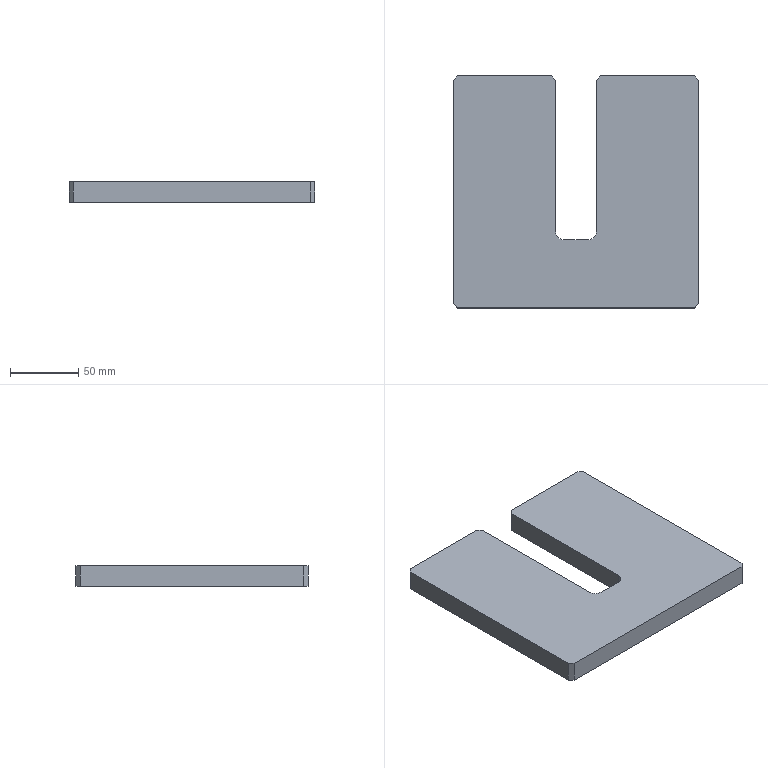Part | STEP file | Planar support platform vertical plate | 1 solid | 18 faces | box 180 x 170 x 15 mm | volume 404827 mm3 | plane 16 | cylinder 2 | commonest cylinder face diameters 12 x2
STEP:
#1=CARTESIAN_POINT('',(0.,0.,0.));
#2=DIRECTION('',(0.,0.,1.));
#3=DIRECTION('',(1.,0.,0.));
#4=AXIS2_PLACEMENT_3D('',#1,#2,#3);
#5=CARTESIAN_POINT('',(87.,85.,15.));
#6=VERTEX_POINT('',#5);
#7=CARTESIAN_POINT('',(18.,85.,15.));
#8=VERTEX_POINT('',#7);
#9=CARTESIAN_POINT('',(15.,85.,15.));
#10=DIRECTION('',(-1.,0.,0.));
#11=VECTOR('',#10,1.);
#12=LINE('',#9,#11);
#13=CARTESIAN_POINT('',(15.,85.,15.));
#14=DIRECTION('',(0.,-1.,0.));
#15=DIRECTION('',(0.,0.,-1.));
#16=AXIS2_PLACEMENT_3D('',#13,#14,#15);
#17=PLANE('',#16);
#18=CARTESIAN_POINT('',(0.,0.));
#19=DIRECTION('',(0.,-1.));
#20=VECTOR('',#19,1.);
#21=LINE('',#18,#20);
#22=(GEOMETRIC_REPRESENTATION_CONTEXT(2)PARAMETRIC_REPRESENTATION_CONTEXT()REPRESENTATION_CONTEXT('',''));
#23=DEFINITIONAL_REPRESENTATION('',(#21),#22);
#24=PCURVE('',#17,#23);
#25=CARTESIAN_POINT('',(0.,0.,15.));
#26=DIRECTION('',(0.,0.,1.));
#27=DIRECTION('',(1.,0.,0.));
#28=AXIS2_PLACEMENT_3D('',#25,#26,#27);
#29=PLANE('',#28);
#30=CARTESIAN_POINT('',(15.,85.));
#31=DIRECTION('',(-1.,0.));
#32=VECTOR('',#31,1.);
#33=LINE('',#30,#32);
#34=(GEOMETRIC_REPRESENTATION_CONTEXT(2)PARAMETRIC_REPRESENTATION_CONTEXT()REPRESENTATION_CONTEXT('',''));
#35=DEFINITIONAL_REPRESENTATION('',(#33),#34);
#36=PCURVE('',#29,#35);
#37=SURFACE_CURVE('',#12,(#24,#36),.PCURVE_S1.);
#38=EDGE_CURVE('',#6,#8,#37,.T.);
#39=ORIENTED_EDGE('',*,*,#38,.F.);
#40=CARTESIAN_POINT('',(87.,85.,0.));
#41=VERTEX_POINT('',#40);
#42=CARTESIAN_POINT('',(87.,85.,15.));
#43=DIRECTION('',(0.,0.,-1.));
#44=VECTOR('',#43,1.);
#45=LINE('',#42,#44);
#46=CARTESIAN_POINT('',(0.,72.));
#47=DIRECTION('',(1.,0.));
#48=VECTOR('',#47,1.);
#49=LINE('',#46,#48);
#50=(GEOMETRIC_REPRESENTATION_CONTEXT(2)PARAMETRIC_REPRESENTATION_CONTEXT()REPRESENTATION_CONTEXT('',''));
#51=DEFINITIONAL_REPRESENTATION('',(#49),#50);
#52=PCURVE('',#17,#51);
#53=CARTESIAN_POINT('',(87.,85.,15.));
#54=DIRECTION('',(-0.7071,-0.7071,0.));
#55=DIRECTION('',(0.,0.,-1.));
#56=AXIS2_PLACEMENT_3D('',#53,#54,#55);
#57=PLANE('',#56);
#58=CARTESIAN_POINT('',(0.,0.));
#59=DIRECTION('',(1.,0.));
#60=VECTOR('',#59,1.);
#61=LINE('',#58,#60);
#62=(GEOMETRIC_REPRESENTATION_CONTEXT(2)PARAMETRIC_REPRESENTATION_CONTEXT()REPRESENTATION_CONTEXT('',''));
#63=DEFINITIONAL_REPRESENTATION('',(#61),#62);
#64=PCURVE('',#57,#63);
#65=SURFACE_CURVE('',#45,(#52,#64),.PCURVE_S1.);
#66=EDGE_CURVE('',#6,#41,#65,.T.);
#67=ORIENTED_EDGE('',*,*,#66,.T.);
#68=CARTESIAN_POINT('',(18.,85.,0.));
#69=VERTEX_POINT('',#68);
#70=CARTESIAN_POINT('',(15.,85.,0.));
#71=DIRECTION('',(-1.,0.,0.));
#72=VECTOR('',#71,1.);
#73=LINE('',#70,#72);
#74=CARTESIAN_POINT('',(15.,0.));
#75=DIRECTION('',(0.,-1.));
#76=VECTOR('',#75,1.);
#77=LINE('',#74,#76);
#78=(GEOMETRIC_REPRESENTATION_CONTEXT(2)PARAMETRIC_REPRESENTATION_CONTEXT()REPRESENTATION_CONTEXT('',''));
#79=DEFINITIONAL_REPRESENTATION('',(#77),#78);
#80=PCURVE('',#17,#79);
#81=CARTESIAN_POINT('',(0.,0.,0.));
#82=DIRECTION('',(0.,0.,1.));
#83=DIRECTION('',(1.,0.,0.));
#84=AXIS2_PLACEMENT_3D('',#81,#82,#83);
#85=PLANE('',#84);
#86=CARTESIAN_POINT('',(15.,85.));
#87=DIRECTION('',(-1.,0.));
#88=VECTOR('',#87,1.);
#89=LINE('',#86,#88);
#90=(GEOMETRIC_REPRESENTATION_CONTEXT(2)PARAMETRIC_REPRESENTATION_CONTEXT()REPRESENTATION_CONTEXT('',''));
#91=DEFINITIONAL_REPRESENTATION('',(#89),#90);
#92=PCURVE('',#85,#91);
#93=SURFACE_CURVE('',#73,(#80,#92),.PCURVE_S1.);
#94=EDGE_CURVE('',#41,#69,#93,.T.);
#95=ORIENTED_EDGE('',*,*,#94,.T.);
#96=CARTESIAN_POINT('',(18.,85.,15.));
#97=DIRECTION('',(0.,0.,1.));
#98=VECTOR('',#97,1.);
#99=LINE('',#96,#98);
#100=CARTESIAN_POINT('',(0.,3.));
#101=DIRECTION('',(-1.,0.));
#102=VECTOR('',#101,1.);
#103=LINE('',#100,#102);
#104=(GEOMETRIC_REPRESENTATION_CONTEXT(2)PARAMETRIC_REPRESENTATION_CONTEXT()REPRESENTATION_CONTEXT('',''));
#105=DEFINITIONAL_REPRESENTATION('',(#103),#104);
#106=PCURVE('',#17,#105);
#107=CARTESIAN_POINT('',(15.,82.,15.));
#108=DIRECTION('',(0.7071,-0.7071,0.));
#109=DIRECTION('',(0.,0.,-1.));
#110=AXIS2_PLACEMENT_3D('',#107,#108,#109);
#111=PLANE('',#110);
#112=CARTESIAN_POINT('',(0.,4.243));
#113=DIRECTION('',(-1.,0.));
#114=VECTOR('',#113,1.);
#115=LINE('',#112,#114);
#116=(GEOMETRIC_REPRESENTATION_CONTEXT(2)PARAMETRIC_REPRESENTATION_CONTEXT()REPRESENTATION_CONTEXT('',''));
#117=DEFINITIONAL_REPRESENTATION('',(#115),#116);
#118=PCURVE('',#111,#117);
#119=SURFACE_CURVE('',#99,(#106,#118),.PCURVE_S1.);
#120=EDGE_CURVE('',#69,#8,#119,.T.);
#121=ORIENTED_EDGE('',*,*,#120,.T.);
#122=EDGE_LOOP('',(#39,#67,#95,#121));
#123=FACE_BOUND('',#122,.T.);
#124=ADVANCED_FACE('',(#123),#17,.F.);
#125=CARTESIAN_POINT('',(15.,82.,15.));
#126=VERTEX_POINT('',#125);
#127=CARTESIAN_POINT('',(15.,-29.,15.));
#128=VERTEX_POINT('',#127);
#129=CARTESIAN_POINT('',(15.,85.,15.));
#130=DIRECTION('',(0.,-1.,0.));
#131=VECTOR('',#130,1.);
#132=LINE('',#129,#131);
#133=CARTESIAN_POINT('',(15.,85.,15.));
#134=DIRECTION('',(1.,0.,0.));
#135=DIRECTION('',(0.,1.,0.));
#136=AXIS2_PLACEMENT_3D('',#133,#134,#135);
#137=PLANE('',#136);
#138=CARTESIAN_POINT('',(0.,0.));
#139=DIRECTION('',(-1.,0.));
#140=VECTOR('',#139,1.);
#141=LINE('',#138,#140);
#142=(GEOMETRIC_REPRESENTATION_CONTEXT(2)PARAMETRIC_REPRESENTATION_CONTEXT()REPRESENTATION_CONTEXT('',''));
#143=DEFINITIONAL_REPRESENTATION('',(#141),#142);
#144=PCURVE('',#137,#143);
#145=CARTESIAN_POINT('',(15.,85.));
#146=DIRECTION('',(0.,-1.));
#147=VECTOR('',#146,1.);
#148=LINE('',#145,#147);
#149=(GEOMETRIC_REPRESENTATION_CONTEXT(2)PARAMETRIC_REPRESENTATION_CONTEXT()REPRESENTATION_CONTEXT('',''));
#150=DEFINITIONAL_REPRESENTATION('',(#148),#149);
#151=PCURVE('',#29,#150);
#152=SURFACE_CURVE('',#132,(#144,#151),.PCURVE_S1.);
#153=EDGE_CURVE('',#126,#128,#152,.T.);
#154=ORIENTED_EDGE('',*,*,#153,.F.);
#155=CARTESIAN_POINT('',(15.,82.,0.));
#156=VERTEX_POINT('',#155);
#157=CARTESIAN_POINT('',(15.,82.,15.));
#158=DIRECTION('',(0.,0.,-1.));
#159=VECTOR('',#158,1.);
#160=LINE('',#157,#159);
#161=CARTESIAN_POINT('',(-3.,0.));
#162=DIRECTION('',(0.,-1.));
#163=VECTOR('',#162,1.);
#164=LINE('',#161,#163);
#165=(GEOMETRIC_REPRESENTATION_CONTEXT(2)PARAMETRIC_REPRESENTATION_CONTEXT()REPRESENTATION_CONTEXT('',''));
#166=DEFINITIONAL_REPRESENTATION('',(#164),#165);
#167=PCURVE('',#137,#166);
#168=CARTESIAN_POINT('',(0.,0.));
#169=DIRECTION('',(1.,0.));
#170=VECTOR('',#169,1.);
#171=LINE('',#168,#170);
#172=(GEOMETRIC_REPRESENTATION_CONTEXT(2)PARAMETRIC_REPRESENTATION_CONTEXT()REPRESENTATION_CONTEXT('',''));
#173=DEFINITIONAL_REPRESENTATION('',(#171),#172);
#174=PCURVE('',#111,#173);
#175=SURFACE_CURVE('',#160,(#167,#174),.PCURVE_S1.);
#176=EDGE_CURVE('',#126,#156,#175,.T.);
#177=ORIENTED_EDGE('',*,*,#176,.T.);
#178=CARTESIAN_POINT('',(15.,-29.,0.));
#179=VERTEX_POINT('',#178);
#180=CARTESIAN_POINT('',(15.,85.,0.));
#181=DIRECTION('',(0.,-1.,0.));
#182=VECTOR('',#181,1.);
#183=LINE('',#180,#182);
#184=CARTESIAN_POINT('',(0.,-15.));
#185=DIRECTION('',(-1.,0.));
#186=VECTOR('',#185,1.);
#187=LINE('',#184,#186);
#188=(GEOMETRIC_REPRESENTATION_CONTEXT(2)PARAMETRIC_REPRESENTATION_CONTEXT()REPRESENTATION_CONTEXT('',''));
#189=DEFINITIONAL_REPRESENTATION('',(#187),#188);
#190=PCURVE('',#137,#189);
#191=CARTESIAN_POINT('',(15.,85.));
#192=DIRECTION('',(0.,-1.));
#193=VECTOR('',#192,1.);
#194=LINE('',#191,#193);
#195=(GEOMETRIC_REPRESENTATION_CONTEXT(2)PARAMETRIC_REPRESENTATION_CONTEXT()REPRESENTATION_CONTEXT('',''));
#196=DEFINITIONAL_REPRESENTATION('',(#194),#195);
#197=PCURVE('',#85,#196);
#198=SURFACE_CURVE('',#183,(#190,#197),.PCURVE_S1.);
#199=EDGE_CURVE('',#156,#179,#198,.T.);
#200=ORIENTED_EDGE('',*,*,#199,.T.);
#201=CARTESIAN_POINT('',(15.,-29.,15.));
#202=DIRECTION('',(0.,0.,1.));
#203=VECTOR('',#202,1.);
#204=LINE('',#201,#203);
#205=CARTESIAN_POINT('',(-114.,0.));
#206=DIRECTION('',(0.,1.));
#207=VECTOR('',#206,1.);
#208=LINE('',#205,#207);
#209=(GEOMETRIC_REPRESENTATION_CONTEXT(2)PARAMETRIC_REPRESENTATION_CONTEXT()REPRESENTATION_CONTEXT('',''));
#210=DEFINITIONAL_REPRESENTATION('',(#208),#209);
#211=PCURVE('',#137,#210);
#212=CARTESIAN_POINT('',(9.,-29.,15.));
#213=DIRECTION('',(0.,0.,1.));
#214=DIRECTION('',(1.,0.,0.));
#215=AXIS2_PLACEMENT_3D('',#212,#213,#214);
#216=CYLINDRICAL_SURFACE('',#215,6.);
#217=CARTESIAN_POINT('',(6.283,0.));
#218=DIRECTION('',(0.,1.));
#219=VECTOR('',#218,1.);
#220=LINE('',#217,#219);
#221=(GEOMETRIC_REPRESENTATION_CONTEXT(2)PARAMETRIC_REPRESENTATION_CONTEXT()REPRESENTATION_CONTEXT('',''));
#222=DEFINITIONAL_REPRESENTATION('',(#220),#221);
#223=PCURVE('',#216,#222);
#224=SURFACE_CURVE('',#204,(#211,#223),.PCURVE_S1.);
#225=EDGE_CURVE('',#179,#128,#224,.T.);
#226=ORIENTED_EDGE('',*,*,#225,.T.);
#227=EDGE_LOOP('',(#154,#177,#200,#226));
#228=FACE_BOUND('',#227,.T.);
#229=ADVANCED_FACE('',(#228),#137,.F.);
#230=CARTESIAN_POINT('',(9.,-35.,15.));
#231=VERTEX_POINT('',#230);
#232=CARTESIAN_POINT('',(-9.,-35.,15.));
#233=VERTEX_POINT('',#232);
#234=CARTESIAN_POINT('',(15.,-35.,15.));
#235=DIRECTION('',(-1.,0.,0.));
#236=VECTOR('',#235,1.);
#237=LINE('',#234,#236);
#238=CARTESIAN_POINT('',(15.,-35.,15.));
#239=DIRECTION('',(0.,-1.,0.));
#240=DIRECTION('',(0.,0.,-1.));
#241=AXIS2_PLACEMENT_3D('',#238,#239,#240);
#242=PLANE('',#241);
#243=CARTESIAN_POINT('',(0.,0.));
#244=DIRECTION('',(0.,-1.));
#245=VECTOR('',#244,1.);
#246=LINE('',#243,#245);
#247=(GEOMETRIC_REPRESENTATION_CONTEXT(2)PARAMETRIC_REPRESENTATION_CONTEXT()REPRESENTATION_CONTEXT('',''));
#248=DEFINITIONAL_REPRESENTATION('',(#246),#247);
#249=PCURVE('',#242,#248);
#250=CARTESIAN_POINT('',(15.,-35.));
#251=DIRECTION('',(-1.,0.));
#252=VECTOR('',#251,1.);
#253=LINE('',#250,#252);
#254=(GEOMETRIC_REPRESENTATION_CONTEXT(2)PARAMETRIC_REPRESENTATION_CONTEXT()REPRESENTATION_CONTEXT('',''));
#255=DEFINITIONAL_REPRESENTATION('',(#253),#254);
#256=PCURVE('',#29,#255);
#257=SURFACE_CURVE('',#237,(#249,#256),.PCURVE_S1.);
#258=EDGE_CURVE('',#231,#233,#257,.T.);
#259=ORIENTED_EDGE('',*,*,#258,.F.);
#260=CARTESIAN_POINT('',(9.,-35.,0.));
#261=VERTEX_POINT('',#260);
#262=CARTESIAN_POINT('',(9.,-35.,0.));
#263=DIRECTION('',(0.,0.,-1.));
#264=VECTOR('',#263,1.);
#265=LINE('',#262,#264);
#266=CARTESIAN_POINT('',(15.,-6.));
#267=DIRECTION('',(1.,0.));
#268=VECTOR('',#267,1.);
#269=LINE('',#266,#268);
#270=(GEOMETRIC_REPRESENTATION_CONTEXT(2)PARAMETRIC_REPRESENTATION_CONTEXT()REPRESENTATION_CONTEXT('',''));
#271=DEFINITIONAL_REPRESENTATION('',(#269),#270);
#272=PCURVE('',#242,#271);
#273=CARTESIAN_POINT('',(4.712,-15.));
#274=DIRECTION('',(0.,-1.));
#275=VECTOR('',#274,1.);
#276=LINE('',#273,#275);
#277=(GEOMETRIC_REPRESENTATION_CONTEXT(2)PARAMETRIC_REPRESENTATION_CONTEXT()REPRESENTATION_CONTEXT('',''));
#278=DEFINITIONAL_REPRESENTATION('',(#276),#277);
#279=PCURVE('',#216,#278);
#280=SURFACE_CURVE('',#265,(#272,#279),.PCURVE_S1.);
#281=EDGE_CURVE('',#231,#261,#280,.T.);
#282=ORIENTED_EDGE('',*,*,#281,.T.);
#283=CARTESIAN_POINT('',(-9.,-35.,0.));
#284=VERTEX_POINT('',#283);
#285=CARTESIAN_POINT('',(15.,-35.,0.));
#286=DIRECTION('',(-1.,0.,0.));
#287=VECTOR('',#286,1.);
#288=LINE('',#285,#287);
#289=CARTESIAN_POINT('',(15.,0.));
#290=DIRECTION('',(0.,-1.));
#291=VECTOR('',#290,1.);
#292=LINE('',#289,#291);
#293=(GEOMETRIC_REPRESENTATION_CONTEXT(2)PARAMETRIC_REPRESENTATION_CONTEXT()REPRESENTATION_CONTEXT('',''));
#294=DEFINITIONAL_REPRESENTATION('',(#292),#293);
#295=PCURVE('',#242,#294);
#296=CARTESIAN_POINT('',(15.,-35.));
#297=DIRECTION('',(-1.,0.));
#298=VECTOR('',#297,1.);
#299=LINE('',#296,#298);
#300=(GEOMETRIC_REPRESENTATION_CONTEXT(2)PARAMETRIC_REPRESENTATION_CONTEXT()REPRESENTATION_CONTEXT('',''));
#301=DEFINITIONAL_REPRESENTATION('',(#299),#300);
#302=PCURVE('',#85,#301);
#303=SURFACE_CURVE('',#288,(#295,#302),.PCURVE_S1.);
#304=EDGE_CURVE('',#261,#284,#303,.T.);
#305=ORIENTED_EDGE('',*,*,#304,.T.);
#306=CARTESIAN_POINT('',(-9.,-35.,15.));
#307=DIRECTION('',(0.,0.,1.));
#308=VECTOR('',#307,1.);
#309=LINE('',#306,#308);
#310=CARTESIAN_POINT('',(0.,-24.));
#311=DIRECTION('',(-1.,0.));
#312=VECTOR('',#311,1.);
#313=LINE('',#310,#312);
#314=(GEOMETRIC_REPRESENTATION_CONTEXT(2)PARAMETRIC_REPRESENTATION_CONTEXT()REPRESENTATION_CONTEXT('',''));
#315=DEFINITIONAL_REPRESENTATION('',(#313),#314);
#316=PCURVE('',#242,#315);
#317=CARTESIAN_POINT('',(-9.,-29.,15.));
#318=DIRECTION('',(0.,0.,1.));
#319=DIRECTION('',(1.,0.,0.));
#320=AXIS2_PLACEMENT_3D('',#317,#318,#319);
#321=CYLINDRICAL_SURFACE('',#320,6.);
#322=CARTESIAN_POINT('',(4.712,0.));
#323=DIRECTION('',(0.,1.));
#324=VECTOR('',#323,1.);
#325=LINE('',#322,#324);
#326=(GEOMETRIC_REPRESENTATION_CONTEXT(2)PARAMETRIC_REPRESENTATION_CONTEXT()REPRESENTATION_CONTEXT('',''));
#327=DEFINITIONAL_REPRESENTATION('',(#325),#326);
#328=PCURVE('',#321,#327);
#329=SURFACE_CURVE('',#309,(#316,#328),.PCURVE_S1.);
#330=EDGE_CURVE('',#284,#233,#329,.T.);
#331=ORIENTED_EDGE('',*,*,#330,.T.);
#332=EDGE_LOOP('',(#259,#282,#305,#331));
#333=FACE_BOUND('',#332,.T.);
#334=ADVANCED_FACE('',(#333),#242,.F.);
#335=CARTESIAN_POINT('',(-15.,-29.,0.));
#336=VERTEX_POINT('',#335);
#337=CARTESIAN_POINT('',(-15.,82.,0.));
#338=VERTEX_POINT('',#337);
#339=CARTESIAN_POINT('',(-15.,85.,0.));
#340=DIRECTION('',(0.,1.,0.));
#341=VECTOR('',#340,1.);
#342=LINE('',#339,#341);
#343=CARTESIAN_POINT('',(-15.,85.,15.));
#344=DIRECTION('',(-1.,0.,0.));
#345=DIRECTION('',(0.,-1.,0.));
#346=AXIS2_PLACEMENT_3D('',#343,#344,#345);
#347=PLANE('',#346);
#348=CARTESIAN_POINT('',(0.,-15.));
#349=DIRECTION('',(-1.,0.));
#350=VECTOR('',#349,1.);
#351=LINE('',#348,#350);
#352=(GEOMETRIC_REPRESENTATION_CONTEXT(2)PARAMETRIC_REPRESENTATION_CONTEXT()REPRESENTATION_CONTEXT('',''));
#353=DEFINITIONAL_REPRESENTATION('',(#351),#352);
#354=PCURVE('',#347,#353);
#355=CARTESIAN_POINT('',(-15.,85.));
#356=DIRECTION('',(0.,1.));
#357=VECTOR('',#356,1.);
#358=LINE('',#355,#357);
#359=(GEOMETRIC_REPRESENTATION_CONTEXT(2)PARAMETRIC_REPRESENTATION_CONTEXT()REPRESENTATION_CONTEXT('',''));
#360=DEFINITIONAL_REPRESENTATION('',(#358),#359);
#361=PCURVE('',#85,#360);
#362=SURFACE_CURVE('',#342,(#354,#361),.PCURVE_S1.);
#363=EDGE_CURVE('',#336,#338,#362,.T.);
#364=ORIENTED_EDGE('',*,*,#363,.T.);
#365=CARTESIAN_POINT('',(-15.,82.,15.));
#366=VERTEX_POINT('',#365);
#367=CARTESIAN_POINT('',(-15.,82.,15.));
#368=DIRECTION('',(0.,0.,1.));
#369=VECTOR('',#368,1.);
#370=LINE('',#367,#369);
#371=CARTESIAN_POINT('',(3.,0.));
#372=DIRECTION('',(0.,1.));
#373=VECTOR('',#372,1.);
#374=LINE('',#371,#373);
#375=(GEOMETRIC_REPRESENTATION_CONTEXT(2)PARAMETRIC_REPRESENTATION_CONTEXT()REPRESENTATION_CONTEXT('',''));
#376=DEFINITIONAL_REPRESENTATION('',(#374),#375);
#377=PCURVE('',#347,#376);
#378=CARTESIAN_POINT('',(-18.,85.,15.));
#379=DIRECTION('',(-0.7071,-0.7071,0.));
#380=DIRECTION('',(0.,0.,-1.));
#381=AXIS2_PLACEMENT_3D('',#378,#379,#380);
#382=PLANE('',#381);
#383=CARTESIAN_POINT('',(0.,4.243));
#384=DIRECTION('',(-1.,0.));
#385=VECTOR('',#384,1.);
#386=LINE('',#383,#385);
#387=(GEOMETRIC_REPRESENTATION_CONTEXT(2)PARAMETRIC_REPRESENTATION_CONTEXT()REPRESENTATION_CONTEXT('',''));
#388=DEFINITIONAL_REPRESENTATION('',(#386),#387);
#389=PCURVE('',#382,#388);
#390=SURFACE_CURVE('',#370,(#377,#389),.PCURVE_S1.);
#391=EDGE_CURVE('',#338,#366,#390,.T.);
#392=ORIENTED_EDGE('',*,*,#391,.T.);
#393=CARTESIAN_POINT('',(-15.,-29.,15.));
#394=VERTEX_POINT('',#393);
#395=CARTESIAN_POINT('',(-15.,85.,15.));
#396=DIRECTION('',(0.,1.,0.));
#397=VECTOR('',#396,1.);
#398=LINE('',#395,#397);
#399=CARTESIAN_POINT('',(0.,0.));
#400=DIRECTION('',(-1.,0.));
#401=VECTOR('',#400,1.);
#402=LINE('',#399,#401);
#403=(GEOMETRIC_REPRESENTATION_CONTEXT(2)PARAMETRIC_REPRESENTATION_CONTEXT()REPRESENTATION_CONTEXT('',''));
#404=DEFINITIONAL_REPRESENTATION('',(#402),#403);
#405=PCURVE('',#347,#404);
#406=CARTESIAN_POINT('',(-15.,85.));
#407=DIRECTION('',(0.,1.));
#408=VECTOR('',#407,1.);
#409=LINE('',#406,#408);
#410=(GEOMETRIC_REPRESENTATION_CONTEXT(2)PARAMETRIC_REPRESENTATION_CONTEXT()REPRESENTATION_CONTEXT('',''));
#411=DEFINITIONAL_REPRESENTATION('',(#409),#410);
#412=PCURVE('',#29,#411);
#413=SURFACE_CURVE('',#398,(#405,#412),.PCURVE_S1.);
#414=EDGE_CURVE('',#394,#366,#413,.T.);
#415=ORIENTED_EDGE('',*,*,#414,.F.);
#416=CARTESIAN_POINT('',(-15.,-29.,0.));
#417=DIRECTION('',(0.,0.,-1.));
#418=VECTOR('',#417,1.);
#419=LINE('',#416,#418);
#420=CARTESIAN_POINT('',(114.,-15.));
#421=DIRECTION('',(0.,-1.));
#422=VECTOR('',#421,1.);
#423=LINE('',#420,#422);
#424=(GEOMETRIC_REPRESENTATION_CONTEXT(2)PARAMETRIC_REPRESENTATION_CONTEXT()REPRESENTATION_CONTEXT('',''));
#425=DEFINITIONAL_REPRESENTATION('',(#423),#424);
#426=PCURVE('',#347,#425);
#427=CARTESIAN_POINT('',(3.142,-15.));
#428=DIRECTION('',(0.,-1.));
#429=VECTOR('',#428,1.);
#430=LINE('',#427,#429);
#431=(GEOMETRIC_REPRESENTATION_CONTEXT(2)PARAMETRIC_REPRESENTATION_CONTEXT()REPRESENTATION_CONTEXT('',''));
#432=DEFINITIONAL_REPRESENTATION('',(#430),#431);
#433=PCURVE('',#321,#432);
#434=SURFACE_CURVE('',#419,(#426,#433),.PCURVE_S1.);
#435=EDGE_CURVE('',#394,#336,#434,.T.);
#436=ORIENTED_EDGE('',*,*,#435,.T.);
#437=EDGE_LOOP('',(#364,#392,#415,#436));
#438=FACE_BOUND('',#437,.T.);
#439=ADVANCED_FACE('',(#438),#347,.F.);
#440=CARTESIAN_POINT('',(-18.,85.,0.));
#441=VERTEX_POINT('',#440);
#442=CARTESIAN_POINT('',(-87.,85.,0.));
#443=VERTEX_POINT('',#442);
#444=CARTESIAN_POINT('',(-90.,85.,0.));
#445=DIRECTION('',(-1.,0.,0.));
#446=VECTOR('',#445,1.);
#447=LINE('',#444,#446);
#448=CARTESIAN_POINT('',(-90.,85.,15.));
#449=DIRECTION('',(0.,-1.,0.));
#450=DIRECTION('',(0.,0.,-1.));
#451=AXIS2_PLACEMENT_3D('',#448,#449,#450);
#452=PLANE('',#451);
#453=CARTESIAN_POINT('',(15.,0.));
#454=DIRECTION('',(0.,-1.));
#455=VECTOR('',#454,1.);
#456=LINE('',#453,#455);
#457=(GEOMETRIC_REPRESENTATION_CONTEXT(2)PARAMETRIC_REPRESENTATION_CONTEXT()REPRESENTATION_CONTEXT('',''));
#458=DEFINITIONAL_REPRESENTATION('',(#456),#457);
#459=PCURVE('',#452,#458);
#460=CARTESIAN_POINT('',(-90.,85.));
#461=DIRECTION('',(-1.,0.));
#462=VECTOR('',#461,1.);
#463=LINE('',#460,#462);
#464=(GEOMETRIC_REPRESENTATION_CONTEXT(2)PARAMETRIC_REPRESENTATION_CONTEXT()REPRESENTATION_CONTEXT('',''));
#465=DEFINITIONAL_REPRESENTATION('',(#463),#464);
#466=PCURVE('',#85,#465);
#467=SURFACE_CURVE('',#447,(#459,#466),.PCURVE_S1.);
#468=EDGE_CURVE('',#441,#443,#467,.T.);
#469=ORIENTED_EDGE('',*,*,#468,.T.);
#470=CARTESIAN_POINT('',(-87.,85.,15.));
#471=VERTEX_POINT('',#470);
#472=CARTESIAN_POINT('',(-87.,85.,15.));
#473=DIRECTION('',(0.,0.,1.));
#474=VECTOR('',#473,1.);
#475=LINE('',#472,#474);
#476=CARTESIAN_POINT('',(0.,3.));
#477=DIRECTION('',(-1.,0.));
#478=VECTOR('',#477,1.);
#479=LINE('',#476,#478);
#480=(GEOMETRIC_REPRESENTATION_CONTEXT(2)PARAMETRIC_REPRESENTATION_CONTEXT()REPRESENTATION_CONTEXT('',''));
#481=DEFINITIONAL_REPRESENTATION('',(#479),#480);
#482=PCURVE('',#452,#481);
#483=CARTESIAN_POINT('',(-90.,82.,15.));
#484=DIRECTION('',(0.7071,-0.7071,0.));
#485=DIRECTION('',(0.,0.,-1.));
#486=AXIS2_PLACEMENT_3D('',#483,#484,#485);
#487=PLANE('',#486);
#488=CARTESIAN_POINT('',(0.,4.243));
#489=DIRECTION('',(-1.,0.));
#490=VECTOR('',#489,1.);
#491=LINE('',#488,#490);
#492=(GEOMETRIC_REPRESENTATION_CONTEXT(2)PARAMETRIC_REPRESENTATION_CONTEXT()REPRESENTATION_CONTEXT('',''));
#493=DEFINITIONAL_REPRESENTATION('',(#491),#492);
#494=PCURVE('',#487,#493);
#495=SURFACE_CURVE('',#475,(#482,#494),.PCURVE_S1.);
#496=EDGE_CURVE('',#443,#471,#495,.T.);
#497=ORIENTED_EDGE('',*,*,#496,.T.);
#498=CARTESIAN_POINT('',(-18.,85.,15.));
#499=VERTEX_POINT('',#498);
#500=CARTESIAN_POINT('',(-90.,85.,15.));
#501=DIRECTION('',(-1.,0.,0.));
#502=VECTOR('',#501,1.);
#503=LINE('',#500,#502);
#504=CARTESIAN_POINT('',(0.,0.));
#505=DIRECTION('',(0.,-1.));
#506=VECTOR('',#505,1.);
#507=LINE('',#504,#506);
#508=(GEOMETRIC_REPRESENTATION_CONTEXT(2)PARAMETRIC_REPRESENTATION_CONTEXT()REPRESENTATION_CONTEXT('',''));
#509=DEFINITIONAL_REPRESENTATION('',(#507),#508);
#510=PCURVE('',#452,#509);
#511=CARTESIAN_POINT('',(-90.,85.));
#512=DIRECTION('',(-1.,0.));
#513=VECTOR('',#512,1.);
#514=LINE('',#511,#513);
#515=(GEOMETRIC_REPRESENTATION_CONTEXT(2)PARAMETRIC_REPRESENTATION_CONTEXT()REPRESENTATION_CONTEXT('',''));
#516=DEFINITIONAL_REPRESENTATION('',(#514),#515);
#517=PCURVE('',#29,#516);
#518=SURFACE_CURVE('',#503,(#510,#517),.PCURVE_S1.);
#519=EDGE_CURVE('',#499,#471,#518,.T.);
#520=ORIENTED_EDGE('',*,*,#519,.F.);
#521=CARTESIAN_POINT('',(-18.,85.,15.));
#522=DIRECTION('',(0.,0.,-1.));
#523=VECTOR('',#522,1.);
#524=LINE('',#521,#523);
#525=CARTESIAN_POINT('',(0.,72.));
#526=DIRECTION('',(1.,0.));
#527=VECTOR('',#526,1.);
#528=LINE('',#525,#527);
#529=(GEOMETRIC_REPRESENTATION_CONTEXT(2)PARAMETRIC_REPRESENTATION_CONTEXT()REPRESENTATION_CONTEXT('',''));
#530=DEFINITIONAL_REPRESENTATION('',(#528),#529);
#531=PCURVE('',#452,#530);
#532=CARTESIAN_POINT('',(0.,0.));
#533=DIRECTION('',(1.,0.));
#534=VECTOR('',#533,1.);
#535=LINE('',#532,#534);
#536=(GEOMETRIC_REPRESENTATION_CONTEXT(2)PARAMETRIC_REPRESENTATION_CONTEXT()REPRESENTATION_CONTEXT('',''));
#537=DEFINITIONAL_REPRESENTATION('',(#535),#536);
#538=PCURVE('',#382,#537);
#539=SURFACE_CURVE('',#524,(#531,#538),.PCURVE_S1.);
#540=EDGE_CURVE('',#499,#441,#539,.T.);
#541=ORIENTED_EDGE('',*,*,#540,.T.);
#542=EDGE_LOOP('',(#469,#497,#520,#541));
#543=FACE_BOUND('',#542,.T.);
#544=ADVANCED_FACE('',(#543),#452,.F.);
#545=CARTESIAN_POINT('',(-90.,82.,0.));
#546=VERTEX_POINT('',#545);
#547=CARTESIAN_POINT('',(-90.,-82.,0.));
#548=VERTEX_POINT('',#547);
#549=CARTESIAN_POINT('',(-90.,-85.,0.));
#550=DIRECTION('',(0.,-1.,0.));
#551=VECTOR('',#550,1.);
#552=LINE('',#549,#551);
#553=CARTESIAN_POINT('',(-90.,-85.,15.));
#554=DIRECTION('',(1.,0.,0.));
#555=DIRECTION('',(0.,0.,-1.));
#556=AXIS2_PLACEMENT_3D('',#553,#554,#555);
#557=PLANE('',#556);
#558=CARTESIAN_POINT('',(15.,0.));
#559=DIRECTION('',(0.,-1.));
#560=VECTOR('',#559,1.);
#561=LINE('',#558,#560);
#562=(GEOMETRIC_REPRESENTATION_CONTEXT(2)PARAMETRIC_REPRESENTATION_CONTEXT()REPRESENTATION_CONTEXT('',''));
#563=DEFINITIONAL_REPRESENTATION('',(#561),#562);
#564=PCURVE('',#557,#563);
#565=CARTESIAN_POINT('',(-90.,-85.));
#566=DIRECTION('',(0.,-1.));
#567=VECTOR('',#566,1.);
#568=LINE('',#565,#567);
#569=(GEOMETRIC_REPRESENTATION_CONTEXT(2)PARAMETRIC_REPRESENTATION_CONTEXT()REPRESENTATION_CONTEXT('',''));
#570=DEFINITIONAL_REPRESENTATION('',(#568),#569);
#571=PCURVE('',#85,#570);
#572=SURFACE_CURVE('',#552,(#564,#571),.PCURVE_S1.);
#573=EDGE_CURVE('',#546,#548,#572,.T.);
#574=ORIENTED_EDGE('',*,*,#573,.T.);
#575=CARTESIAN_POINT('',(-90.,-82.,15.));
#576=VERTEX_POINT('',#575);
#577=CARTESIAN_POINT('',(-90.,-82.,15.));
#578=DIRECTION('',(0.,0.,1.));
#579=VECTOR('',#578,1.);
#580=LINE('',#577,#579);
#581=CARTESIAN_POINT('',(0.,3.));
#582=DIRECTION('',(-1.,0.));
#583=VECTOR('',#582,1.);
#584=LINE('',#581,#583);
#585=(GEOMETRIC_REPRESENTATION_CONTEXT(2)PARAMETRIC_REPRESENTATION_CONTEXT()REPRESENTATION_CONTEXT('',''));
#586=DEFINITIONAL_REPRESENTATION('',(#584),#585);
#587=PCURVE('',#557,#586);
#588=CARTESIAN_POINT('',(-87.,-85.,15.));
#589=DIRECTION('',(0.7071,0.7071,0.));
#590=DIRECTION('',(0.,0.,-1.));
#591=AXIS2_PLACEMENT_3D('',#588,#589,#590);
#592=PLANE('',#591);
#593=CARTESIAN_POINT('',(0.,4.243));
#594=DIRECTION('',(-1.,0.));
#595=VECTOR('',#594,1.);
#596=LINE('',#593,#595);
#597=(GEOMETRIC_REPRESENTATION_CONTEXT(2)PARAMETRIC_REPRESENTATION_CONTEXT()REPRESENTATION_CONTEXT('',''));
#598=DEFINITIONAL_REPRESENTATION('',(#596),#597);
#599=PCURVE('',#592,#598);
#600=SURFACE_CURVE('',#580,(#587,#599),.PCURVE_S1.);
#601=EDGE_CURVE('',#548,#576,#600,.T.);
#602=ORIENTED_EDGE('',*,*,#601,.T.);
#603=CARTESIAN_POINT('',(-90.,82.,15.));
#604=VERTEX_POINT('',#603);
#605=CARTESIAN_POINT('',(-90.,-85.,15.));
#606=DIRECTION('',(0.,-1.,0.));
#607=VECTOR('',#606,1.);
#608=LINE('',#605,#607);
#609=CARTESIAN_POINT('',(0.,0.));
#610=DIRECTION('',(0.,-1.));
#611=VECTOR('',#610,1.);
#612=LINE('',#609,#611);
#613=(GEOMETRIC_REPRESENTATION_CONTEXT(2)PARAMETRIC_REPRESENTATION_CONTEXT()REPRESENTATION_CONTEXT('',''));
#614=DEFINITIONAL_REPRESENTATION('',(#612),#613);
#615=PCURVE('',#557,#614);
#616=CARTESIAN_POINT('',(-90.,-85.));
#617=DIRECTION('',(0.,-1.));
#618=VECTOR('',#617,1.);
#619=LINE('',#616,#618);
#620=(GEOMETRIC_REPRESENTATION_CONTEXT(2)PARAMETRIC_REPRESENTATION_CONTEXT()REPRESENTATION_CONTEXT('',''));
#621=DEFINITIONAL_REPRESENTATION('',(#619),#620);
#622=PCURVE('',#29,#621);
#623=SURFACE_CURVE('',#608,(#615,#622),.PCURVE_S1.);
#624=EDGE_CURVE('',#604,#576,#623,.T.);
#625=ORIENTED_EDGE('',*,*,#624,.F.);
#626=CARTESIAN_POINT('',(-90.,82.,15.));
#627=DIRECTION('',(0.,0.,-1.));
#628=VECTOR('',#627,1.);
#629=LINE('',#626,#628);
#630=CARTESIAN_POINT('',(0.,167.));
#631=DIRECTION('',(1.,0.));
#632=VECTOR('',#631,1.);
#633=LINE('',#630,#632);
#634=(GEOMETRIC_REPRESENTATION_CONTEXT(2)PARAMETRIC_REPRESENTATION_CONTEXT()REPRESENTATION_CONTEXT('',''));
#635=DEFINITIONAL_REPRESENTATION('',(#633),#634);
#636=PCURVE('',#557,#635);
#637=CARTESIAN_POINT('',(0.,0.));
#638=DIRECTION('',(1.,0.));
#639=VECTOR('',#638,1.);
#640=LINE('',#637,#639);
#641=(GEOMETRIC_REPRESENTATION_CONTEXT(2)PARAMETRIC_REPRESENTATION_CONTEXT()REPRESENTATION_CONTEXT('',''));
#642=DEFINITIONAL_REPRESENTATION('',(#640),#641);
#643=PCURVE('',#487,#642);
#644=SURFACE_CURVE('',#629,(#636,#643),.PCURVE_S1.);
#645=EDGE_CURVE('',#604,#546,#644,.T.);
#646=ORIENTED_EDGE('',*,*,#645,.T.);
#647=EDGE_LOOP('',(#574,#602,#625,#646));
#648=FACE_BOUND('',#647,.T.);
#649=ADVANCED_FACE('',(#648),#557,.F.);
#650=CARTESIAN_POINT('',(-87.,-85.,0.));
#651=VERTEX_POINT('',#650);
#652=CARTESIAN_POINT('',(87.,-85.,0.));
#653=VERTEX_POINT('',#652);
#654=CARTESIAN_POINT('',(-90.,-85.,0.));
#655=DIRECTION('',(1.,0.,0.));
#656=VECTOR('',#655,1.);
#657=LINE('',#654,#656);
#658=CARTESIAN_POINT('',(-90.,-85.,15.));
#659=DIRECTION('',(0.,1.,0.));
#660=DIRECTION('',(0.,0.,1.));
#661=AXIS2_PLACEMENT_3D('',#658,#659,#660);
#662=PLANE('',#661);
#663=CARTESIAN_POINT('',(-15.,0.));
#664=DIRECTION('',(0.,1.));
#665=VECTOR('',#664,1.);
#666=LINE('',#663,#665);
#667=(GEOMETRIC_REPRESENTATION_CONTEXT(2)PARAMETRIC_REPRESENTATION_CONTEXT()REPRESENTATION_CONTEXT('',''));
#668=DEFINITIONAL_REPRESENTATION('',(#666),#667);
#669=PCURVE('',#662,#668);
#670=CARTESIAN_POINT('',(-90.,-85.));
#671=DIRECTION('',(1.,0.));
#672=VECTOR('',#671,1.);
#673=LINE('',#670,#672);
#674=(GEOMETRIC_REPRESENTATION_CONTEXT(2)PARAMETRIC_REPRESENTATION_CONTEXT()REPRESENTATION_CONTEXT('',''));
#675=DEFINITIONAL_REPRESENTATION('',(#673),#674);
#676=PCURVE('',#85,#675);
#677=SURFACE_CURVE('',#657,(#669,#676),.PCURVE_S1.);
#678=EDGE_CURVE('',#651,#653,#677,.T.);
#679=ORIENTED_EDGE('',*,*,#678,.T.);
#680=CARTESIAN_POINT('',(87.,-85.,15.));
#681=VERTEX_POINT('',#680);
#682=CARTESIAN_POINT('',(87.,-85.,15.));
#683=DIRECTION('',(0.,0.,1.));
#684=VECTOR('',#683,1.);
#685=LINE('',#682,#684);
#686=CARTESIAN_POINT('',(0.,177.));
#687=DIRECTION('',(1.,0.));
#688=VECTOR('',#687,1.);
#689=LINE('',#686,#688);
#690=(GEOMETRIC_REPRESENTATION_CONTEXT(2)PARAMETRIC_REPRESENTATION_CONTEXT()REPRESENTATION_CONTEXT('',''));
#691=DEFINITIONAL_REPRESENTATION('',(#689),#690);
#692=PCURVE('',#662,#691);
#693=CARTESIAN_POINT('',(90.,-82.,15.));
#694=DIRECTION('',(-0.7071,0.7071,0.));
#695=DIRECTION('',(0.,0.,-1.));
#696=AXIS2_PLACEMENT_3D('',#693,#694,#695);
#697=PLANE('',#696);
#698=CARTESIAN_POINT('',(0.,4.243));
#699=DIRECTION('',(-1.,0.));
#700=VECTOR('',#699,1.);
#701=LINE('',#698,#700);
#702=(GEOMETRIC_REPRESENTATION_CONTEXT(2)PARAMETRIC_REPRESENTATION_CONTEXT()REPRESENTATION_CONTEXT('',''));
#703=DEFINITIONAL_REPRESENTATION('',(#701),#702);
#704=PCURVE('',#697,#703);
#705=SURFACE_CURVE('',#685,(#692,#704),.PCURVE_S1.);
#706=EDGE_CURVE('',#653,#681,#705,.T.);
#707=ORIENTED_EDGE('',*,*,#706,.T.);
#708=CARTESIAN_POINT('',(-87.,-85.,15.));
#709=VERTEX_POINT('',#708);
#710=CARTESIAN_POINT('',(-90.,-85.,15.));
#711=DIRECTION('',(1.,0.,0.));
#712=VECTOR('',#711,1.);
#713=LINE('',#710,#712);
#714=CARTESIAN_POINT('',(0.,0.));
#715=DIRECTION('',(0.,1.));
#716=VECTOR('',#715,1.);
#717=LINE('',#714,#716);
#718=(GEOMETRIC_REPRESENTATION_CONTEXT(2)PARAMETRIC_REPRESENTATION_CONTEXT()REPRESENTATION_CONTEXT('',''));
#719=DEFINITIONAL_REPRESENTATION('',(#717),#718);
#720=PCURVE('',#662,#719);
#721=CARTESIAN_POINT('',(-90.,-85.));
#722=DIRECTION('',(1.,0.));
#723=VECTOR('',#722,1.);
#724=LINE('',#721,#723);
#725=(GEOMETRIC_REPRESENTATION_CONTEXT(2)PARAMETRIC_REPRESENTATION_CONTEXT()REPRESENTATION_CONTEXT('',''));
#726=DEFINITIONAL_REPRESENTATION('',(#724),#725);
#727=PCURVE('',#29,#726);
#728=SURFACE_CURVE('',#713,(#720,#727),.PCURVE_S1.);
#729=EDGE_CURVE('',#709,#681,#728,.T.);
#730=ORIENTED_EDGE('',*,*,#729,.F.);
#731=CARTESIAN_POINT('',(-87.,-85.,15.));
#732=DIRECTION('',(0.,0.,-1.));
#733=VECTOR('',#732,1.);
#734=LINE('',#731,#733);
#735=CARTESIAN_POINT('',(0.,3.));
#736=DIRECTION('',(-1.,0.));
#737=VECTOR('',#736,1.);
#738=LINE('',#735,#737);
#739=(GEOMETRIC_REPRESENTATION_CONTEXT(2)PARAMETRIC_REPRESENTATION_CONTEXT()REPRESENTATION_CONTEXT('',''));
#740=DEFINITIONAL_REPRESENTATION('',(#738),#739);
#741=PCURVE('',#662,#740);
#742=CARTESIAN_POINT('',(0.,0.));
#743=DIRECTION('',(1.,0.));
#744=VECTOR('',#743,1.);
#745=LINE('',#742,#744);
#746=(GEOMETRIC_REPRESENTATION_CONTEXT(2)PARAMETRIC_REPRESENTATION_CONTEXT()REPRESENTATION_CONTEXT('',''));
#747=DEFINITIONAL_REPRESENTATION('',(#745),#746);
#748=PCURVE('',#592,#747);
#749=SURFACE_CURVE('',#734,(#741,#748),.PCURVE_S1.);
#750=EDGE_CURVE('',#709,#651,#749,.T.);
#751=ORIENTED_EDGE('',*,*,#750,.T.);
#752=EDGE_LOOP('',(#679,#707,#730,#751));
#753=FACE_BOUND('',#752,.T.);
#754=ADVANCED_FACE('',(#753),#662,.F.);
#755=CARTESIAN_POINT('',(90.,-82.,0.));
#756=VERTEX_POINT('',#755);
#757=CARTESIAN_POINT('',(90.,82.,0.));
#758=VERTEX_POINT('',#757);
#759=CARTESIAN_POINT('',(90.,-85.,0.));
#760=DIRECTION('',(0.,1.,0.));
#761=VECTOR('',#760,1.);
#762=LINE('',#759,#761);
#763=CARTESIAN_POINT('',(90.,-85.,15.));
#764=DIRECTION('',(-1.,0.,0.));
#765=DIRECTION('',(0.,0.,1.));
#766=AXIS2_PLACEMENT_3D('',#763,#764,#765);
#767=PLANE('',#766);
#768=CARTESIAN_POINT('',(-15.,0.));
#769=DIRECTION('',(0.,1.));
#770=VECTOR('',#769,1.);
#771=LINE('',#768,#770);
#772=(GEOMETRIC_REPRESENTATION_CONTEXT(2)PARAMETRIC_REPRESENTATION_CONTEXT()REPRESENTATION_CONTEXT('',''));
#773=DEFINITIONAL_REPRESENTATION('',(#771),#772);
#774=PCURVE('',#767,#773);
#775=CARTESIAN_POINT('',(90.,-85.));
#776=DIRECTION('',(0.,1.));
#777=VECTOR('',#776,1.);
#778=LINE('',#775,#777);
#779=(GEOMETRIC_REPRESENTATION_CONTEXT(2)PARAMETRIC_REPRESENTATION_CONTEXT()REPRESENTATION_CONTEXT('',''));
#780=DEFINITIONAL_REPRESENTATION('',(#778),#779);
#781=PCURVE('',#85,#780);
#782=SURFACE_CURVE('',#762,(#774,#781),.PCURVE_S1.);
#783=EDGE_CURVE('',#756,#758,#782,.T.);
#784=ORIENTED_EDGE('',*,*,#783,.T.);
#785=CARTESIAN_POINT('',(90.,82.,15.));
#786=VERTEX_POINT('',#785);
#787=CARTESIAN_POINT('',(90.,82.,15.));
#788=DIRECTION('',(0.,0.,1.));
#789=VECTOR('',#788,1.);
#790=LINE('',#787,#789);
#791=CARTESIAN_POINT('',(0.,167.));
#792=DIRECTION('',(1.,0.));
#793=VECTOR('',#792,1.);
#794=LINE('',#791,#793);
#795=(GEOMETRIC_REPRESENTATION_CONTEXT(2)PARAMETRIC_REPRESENTATION_CONTEXT()REPRESENTATION_CONTEXT('',''));
#796=DEFINITIONAL_REPRESENTATION('',(#794),#795);
#797=PCURVE('',#767,#796);
#798=CARTESIAN_POINT('',(0.,4.243));
#799=DIRECTION('',(-1.,0.));
#800=VECTOR('',#799,1.);
#801=LINE('',#798,#800);
#802=(GEOMETRIC_REPRESENTATION_CONTEXT(2)PARAMETRIC_REPRESENTATION_CONTEXT()REPRESENTATION_CONTEXT('',''));
#803=DEFINITIONAL_REPRESENTATION('',(#801),#802);
#804=PCURVE('',#57,#803);
#805=SURFACE_CURVE('',#790,(#797,#804),.PCURVE_S1.);
#806=EDGE_CURVE('',#758,#786,#805,.T.);
#807=ORIENTED_EDGE('',*,*,#806,.T.);
#808=CARTESIAN_POINT('',(90.,-82.,15.));
#809=VERTEX_POINT('',#808);
#810=CARTESIAN_POINT('',(90.,-85.,15.));
#811=DIRECTION('',(0.,1.,0.));
#812=VECTOR('',#811,1.);
#813=LINE('',#810,#812);
#814=CARTESIAN_POINT('',(0.,0.));
#815=DIRECTION('',(0.,1.));
#816=VECTOR('',#815,1.);
#817=LINE('',#814,#816);
#818=(GEOMETRIC_REPRESENTATION_CONTEXT(2)PARAMETRIC_REPRESENTATION_CONTEXT()REPRESENTATION_CONTEXT('',''));
#819=DEFINITIONAL_REPRESENTATION('',(#817),#818);
#820=PCURVE('',#767,#819);
#821=CARTESIAN_POINT('',(90.,-85.));
#822=DIRECTION('',(0.,1.));
#823=VECTOR('',#822,1.);
#824=LINE('',#821,#823);
#825=(GEOMETRIC_REPRESENTATION_CONTEXT(2)PARAMETRIC_REPRESENTATION_CONTEXT()REPRESENTATION_CONTEXT('',''));
#826=DEFINITIONAL_REPRESENTATION('',(#824),#825);
#827=PCURVE('',#29,#826);
#828=SURFACE_CURVE('',#813,(#820,#827),.PCURVE_S1.);
#829=EDGE_CURVE('',#809,#786,#828,.T.);
#830=ORIENTED_EDGE('',*,*,#829,.F.);
#831=CARTESIAN_POINT('',(90.,-82.,15.));
#832=DIRECTION('',(0.,0.,-1.));
#833=VECTOR('',#832,1.);
#834=LINE('',#831,#833);
#835=CARTESIAN_POINT('',(0.,3.));
#836=DIRECTION('',(-1.,0.));
#837=VECTOR('',#836,1.);
#838=LINE('',#835,#837);
#839=(GEOMETRIC_REPRESENTATION_CONTEXT(2)PARAMETRIC_REPRESENTATION_CONTEXT()REPRESENTATION_CONTEXT('',''));
#840=DEFINITIONAL_REPRESENTATION('',(#838),#839);
#841=PCURVE('',#767,#840);
#842=CARTESIAN_POINT('',(0.,0.));
#843=DIRECTION('',(1.,0.));
#844=VECTOR('',#843,1.);
#845=LINE('',#842,#844);
#846=(GEOMETRIC_REPRESENTATION_CONTEXT(2)PARAMETRIC_REPRESENTATION_CONTEXT()REPRESENTATION_CONTEXT('',''));
#847=DEFINITIONAL_REPRESENTATION('',(#845),#846);
#848=PCURVE('',#697,#847);
#849=SURFACE_CURVE('',#834,(#841,#848),.PCURVE_S1.);
#850=EDGE_CURVE('',#809,#756,#849,.T.);
#851=ORIENTED_EDGE('',*,*,#850,.T.);
#852=EDGE_LOOP('',(#784,#807,#830,#851));
#853=FACE_BOUND('',#852,.T.);
#854=ADVANCED_FACE('',(#853),#767,.F.);
#855=ORIENTED_EDGE('',*,*,#829,.T.);
#856=CARTESIAN_POINT('',(86.,86.,15.));
#857=DIRECTION('',(-0.7071,0.7071,0.));
#858=VECTOR('',#857,1.);
#859=LINE('',#856,#858);
#860=CARTESIAN_POINT('',(86.,86.));
#861=DIRECTION('',(-0.7071,0.7071));
#862=VECTOR('',#861,1.);
#863=LINE('',#860,#862);
#864=(GEOMETRIC_REPRESENTATION_CONTEXT(2)PARAMETRIC_REPRESENTATION_CONTEXT()REPRESENTATION_CONTEXT('',''));
#865=DEFINITIONAL_REPRESENTATION('',(#863),#864);
#866=PCURVE('',#29,#865);
#867=CARTESIAN_POINT('',(0.,-1.414));
#868=DIRECTION('',(0.,-1.));
#869=VECTOR('',#868,1.);
#870=LINE('',#867,#869);
#871=(GEOMETRIC_REPRESENTATION_CONTEXT(2)PARAMETRIC_REPRESENTATION_CONTEXT()REPRESENTATION_CONTEXT('',''));
#872=DEFINITIONAL_REPRESENTATION('',(#870),#871);
#873=PCURVE('',#57,#872);
#874=SURFACE_CURVE('',#859,(#866,#873),.PCURVE_S1.);
#875=EDGE_CURVE('',#786,#6,#874,.T.);
#876=ORIENTED_EDGE('',*,*,#875,.T.);
#877=ORIENTED_EDGE('',*,*,#38,.T.);
#878=CARTESIAN_POINT('',(-33.5,33.5,15.));
#879=DIRECTION('',(-0.7071,-0.7071,0.));
#880=VECTOR('',#879,1.);
#881=LINE('',#878,#880);
#882=CARTESIAN_POINT('',(-33.5,33.5));
#883=DIRECTION('',(-0.7071,-0.7071));
#884=VECTOR('',#883,1.);
#885=LINE('',#882,#884);
#886=(GEOMETRIC_REPRESENTATION_CONTEXT(2)PARAMETRIC_REPRESENTATION_CONTEXT()REPRESENTATION_CONTEXT('',''));
#887=DEFINITIONAL_REPRESENTATION('',(#885),#886);
#888=PCURVE('',#29,#887);
#889=CARTESIAN_POINT('',(0.,-68.589));
#890=DIRECTION('',(0.,-1.));
#891=VECTOR('',#890,1.);
#892=LINE('',#889,#891);
#893=(GEOMETRIC_REPRESENTATION_CONTEXT(2)PARAMETRIC_REPRESENTATION_CONTEXT()REPRESENTATION_CONTEXT('',''));
#894=DEFINITIONAL_REPRESENTATION('',(#892),#893);
#895=PCURVE('',#111,#894);
#896=SURFACE_CURVE('',#881,(#888,#895),.PCURVE_S1.);
#897=EDGE_CURVE('',#8,#126,#896,.T.);
#898=ORIENTED_EDGE('',*,*,#897,.T.);
#899=ORIENTED_EDGE('',*,*,#153,.T.);
#900=CARTESIAN_POINT('',(9.,-29.,15.));
#901=DIRECTION('',(0.,0.,-1.));
#902=DIRECTION('',(1.,0.,0.));
#903=AXIS2_PLACEMENT_3D('',#900,#901,#902);
#904=CIRCLE('',#903,6.);
#905=CARTESIAN_POINT('',(15.,-29.));
#906=CARTESIAN_POINT('',(15.,-39.392));
#907=CARTESIAN_POINT('',(6.,-34.196));
#908=CARTESIAN_POINT('',(-3.,-29.));
#909=CARTESIAN_POINT('',(6.,-23.804));
#910=CARTESIAN_POINT('',(15.,-18.608));
#911=CARTESIAN_POINT('',(15.,-29.));
#912=(BOUNDED_CURVE()B_SPLINE_CURVE(2,(#905,#906,#907,#908,#909,#910,#911),.UNSPECIFIED.,.T.,.F.)B_SPLINE_CURVE_WITH_KNOTS((1,2,2,2,2,1),(-2.094,0.,2.094,4.189,6.283,8.378),.UNSPECIFIED.)CURVE()GEOMETRIC_REPRESENTATION_ITEM()RATIONAL_B_SPLINE_CURVE((1.,0.5,1.,0.5,1.,0.5,1.))REPRESENTATION_ITEM(''));
#913=(GEOMETRIC_REPRESENTATION_CONTEXT(2)PARAMETRIC_REPRESENTATION_CONTEXT()REPRESENTATION_CONTEXT('',''));
#914=DEFINITIONAL_REPRESENTATION('',(#912),#913);
#915=PCURVE('',#29,#914);
#916=CARTESIAN_POINT('',(6.283,0.));
#917=DIRECTION('',(-1.,0.));
#918=VECTOR('',#917,1.);
#919=LINE('',#916,#918);
#920=(GEOMETRIC_REPRESENTATION_CONTEXT(2)PARAMETRIC_REPRESENTATION_CONTEXT()REPRESENTATION_CONTEXT('',''));
#921=DEFINITIONAL_REPRESENTATION('',(#919),#920);
#922=PCURVE('',#216,#921);
#923=SURFACE_CURVE('',#904,(#915,#922),.PCURVE_S1.);
#924=EDGE_CURVE('',#128,#231,#923,.T.);
#925=ORIENTED_EDGE('',*,*,#924,.T.);
#926=ORIENTED_EDGE('',*,*,#258,.T.);
#927=CARTESIAN_POINT('',(-9.,-29.,15.));
#928=DIRECTION('',(0.,0.,-1.));
#929=DIRECTION('',(1.,0.,0.));
#930=AXIS2_PLACEMENT_3D('',#927,#928,#929);
#931=CIRCLE('',#930,6.);
#932=CARTESIAN_POINT('',(-3.,-29.));
#933=CARTESIAN_POINT('',(-3.,-39.392));
#934=CARTESIAN_POINT('',(-12.,-34.196));
#935=CARTESIAN_POINT('',(-21.,-29.));
#936=CARTESIAN_POINT('',(-12.,-23.804));
#937=CARTESIAN_POINT('',(-3.,-18.608));
#938=CARTESIAN_POINT('',(-3.,-29.));
#939=(BOUNDED_CURVE()B_SPLINE_CURVE(2,(#932,#933,#934,#935,#936,#937,#938),.UNSPECIFIED.,.T.,.F.)B_SPLINE_CURVE_WITH_KNOTS((1,2,2,2,2,1),(-2.094,0.,2.094,4.189,6.283,8.378),.UNSPECIFIED.)CURVE()GEOMETRIC_REPRESENTATION_ITEM()RATIONAL_B_SPLINE_CURVE((1.,0.5,1.,0.5,1.,0.5,1.))REPRESENTATION_ITEM(''));
#940=(GEOMETRIC_REPRESENTATION_CONTEXT(2)PARAMETRIC_REPRESENTATION_CONTEXT()REPRESENTATION_CONTEXT('',''));
#941=DEFINITIONAL_REPRESENTATION('',(#939),#940);
#942=PCURVE('',#29,#941);
#943=CARTESIAN_POINT('',(6.283,0.));
#944=DIRECTION('',(-1.,0.));
#945=VECTOR('',#944,1.);
#946=LINE('',#943,#945);
#947=(GEOMETRIC_REPRESENTATION_CONTEXT(2)PARAMETRIC_REPRESENTATION_CONTEXT()REPRESENTATION_CONTEXT('',''));
#948=DEFINITIONAL_REPRESENTATION('',(#946),#947);
#949=PCURVE('',#321,#948);
#950=SURFACE_CURVE('',#931,(#942,#949),.PCURVE_S1.);
#951=EDGE_CURVE('',#233,#394,#950,.T.);
#952=ORIENTED_EDGE('',*,*,#951,.T.);
#953=ORIENTED_EDGE('',*,*,#414,.T.);
#954=CARTESIAN_POINT('',(33.5,33.5,15.));
#955=DIRECTION('',(-0.7071,0.7071,0.));
#956=VECTOR('',#955,1.);
#957=LINE('',#954,#956);
#958=CARTESIAN_POINT('',(33.5,33.5));
#959=DIRECTION('',(-0.7071,0.7071));
#960=VECTOR('',#959,1.);
#961=LINE('',#958,#960);
#962=(GEOMETRIC_REPRESENTATION_CONTEXT(2)PARAMETRIC_REPRESENTATION_CONTEXT()REPRESENTATION_CONTEXT('',''));
#963=DEFINITIONAL_REPRESENTATION('',(#961),#962);
#964=PCURVE('',#29,#963);
#965=CARTESIAN_POINT('',(0.,72.832));
#966=DIRECTION('',(0.,-1.));
#967=VECTOR('',#966,1.);
#968=LINE('',#965,#967);
#969=(GEOMETRIC_REPRESENTATION_CONTEXT(2)PARAMETRIC_REPRESENTATION_CONTEXT()REPRESENTATION_CONTEXT('',''));
#970=DEFINITIONAL_REPRESENTATION('',(#968),#969);
#971=PCURVE('',#382,#970);
#972=SURFACE_CURVE('',#957,(#964,#971),.PCURVE_S1.);
#973=EDGE_CURVE('',#366,#499,#972,.T.);
#974=ORIENTED_EDGE('',*,*,#973,.T.);
#975=ORIENTED_EDGE('',*,*,#519,.T.);
#976=CARTESIAN_POINT('',(-86.,86.,15.));
#977=DIRECTION('',(-0.7071,-0.7071,0.));
#978=VECTOR('',#977,1.);
#979=LINE('',#976,#978);
#980=CARTESIAN_POINT('',(-86.,86.));
#981=DIRECTION('',(-0.7071,-0.7071));
#982=VECTOR('',#981,1.);
#983=LINE('',#980,#982);
#984=(GEOMETRIC_REPRESENTATION_CONTEXT(2)PARAMETRIC_REPRESENTATION_CONTEXT()REPRESENTATION_CONTEXT('',''));
#985=DEFINITIONAL_REPRESENTATION('',(#983),#984);
#986=PCURVE('',#29,#985);
#987=CARTESIAN_POINT('',(0.,5.657));
#988=DIRECTION('',(0.,-1.));
#989=VECTOR('',#988,1.);
#990=LINE('',#987,#989);
#991=(GEOMETRIC_REPRESENTATION_CONTEXT(2)PARAMETRIC_REPRESENTATION_CONTEXT()REPRESENTATION_CONTEXT('',''));
#992=DEFINITIONAL_REPRESENTATION('',(#990),#991);
#993=PCURVE('',#487,#992);
#994=SURFACE_CURVE('',#979,(#986,#993),.PCURVE_S1.);
#995=EDGE_CURVE('',#471,#604,#994,.T.);
#996=ORIENTED_EDGE('',*,*,#995,.T.);
#997=ORIENTED_EDGE('',*,*,#624,.T.);
#998=CARTESIAN_POINT('',(-86.,-86.,15.));
#999=DIRECTION('',(0.7071,-0.7071,0.));
#1000=VECTOR('',#999,1.);
#1001=LINE('',#998,#1000);
#1002=CARTESIAN_POINT('',(-86.,-86.));
#1003=DIRECTION('',(0.7071,-0.7071));
#1004=VECTOR('',#1003,1.);
#1005=LINE('',#1002,#1004);
#1006=(GEOMETRIC_REPRESENTATION_CONTEXT(2)PARAMETRIC_REPRESENTATION_CONTEXT()REPRESENTATION_CONTEXT('',''));
#1007=DEFINITIONAL_REPRESENTATION('',(#1005),#1006);
#1008=PCURVE('',#29,#1007);
#1009=CARTESIAN_POINT('',(0.,-1.414));
#1010=DIRECTION('',(0.,-1.));
#1011=VECTOR('',#1010,1.);
#1012=LINE('',#1009,#1011);
#1013=(GEOMETRIC_REPRESENTATION_CONTEXT(2)PARAMETRIC_REPRESENTATION_CONTEXT()REPRESENTATION_CONTEXT('',''));
#1014=DEFINITIONAL_REPRESENTATION('',(#1012),#1013);
#1015=PCURVE('',#592,#1014);
#1016=SURFACE_CURVE('',#1001,(#1008,#1015),.PCURVE_S1.);
#1017=EDGE_CURVE('',#576,#709,#1016,.T.);
#1018=ORIENTED_EDGE('',*,*,#1017,.T.);
#1019=ORIENTED_EDGE('',*,*,#729,.T.);
#1020=CARTESIAN_POINT('',(86.,-86.,15.));
#1021=DIRECTION('',(0.7071,0.7071,0.));
#1022=VECTOR('',#1021,1.);
#1023=LINE('',#1020,#1022);
#1024=CARTESIAN_POINT('',(86.,-86.));
#1025=DIRECTION('',(0.7071,0.7071));
#1026=VECTOR('',#1025,1.);
#1027=LINE('',#1024,#1026);
#1028=(GEOMETRIC_REPRESENTATION_CONTEXT(2)PARAMETRIC_REPRESENTATION_CONTEXT()REPRESENTATION_CONTEXT('',''));
#1029=DEFINITIONAL_REPRESENTATION('',(#1027),#1028);
#1030=PCURVE('',#29,#1029);
#1031=CARTESIAN_POINT('',(0.,5.657));
#1032=DIRECTION('',(0.,-1.));
#1033=VECTOR('',#1032,1.);
#1034=LINE('',#1031,#1033);
#1035=(GEOMETRIC_REPRESENTATION_CONTEXT(2)PARAMETRIC_REPRESENTATION_CONTEXT()REPRESENTATION_CONTEXT('',''));
#1036=DEFINITIONAL_REPRESENTATION('',(#1034),#1035);
#1037=PCURVE('',#697,#1036);
#1038=SURFACE_CURVE('',#1023,(#1030,#1037),.PCURVE_S1.);
#1039=EDGE_CURVE('',#681,#809,#1038,.T.);
#1040=ORIENTED_EDGE('',*,*,#1039,.T.);
#1041=EDGE_LOOP('',(#855,#876,#877,#898,#899,#925,#926,#952,#953,#974,#975,#996,#997,#1018,#1019,#1040));
#1042=FACE_BOUND('',#1041,.T.);
#1043=ADVANCED_FACE('',(#1042),#29,.T.);
#1044=ORIENTED_EDGE('',*,*,#94,.F.);
#1045=CARTESIAN_POINT('',(87.,85.,0.));
#1046=DIRECTION('',(0.7071,-0.7071,0.));
#1047=VECTOR('',#1046,1.);
#1048=LINE('',#1045,#1047);
#1049=CARTESIAN_POINT('',(87.,85.));
#1050=DIRECTION('',(0.7071,-0.7071));
#1051=VECTOR('',#1050,1.);
#1052=LINE('',#1049,#1051);
#1053=(GEOMETRIC_REPRESENTATION_CONTEXT(2)PARAMETRIC_REPRESENTATION_CONTEXT()REPRESENTATION_CONTEXT('',''));
#1054=DEFINITIONAL_REPRESENTATION('',(#1052),#1053);
#1055=PCURVE('',#85,#1054);
#1056=CARTESIAN_POINT('',(15.,0.));
#1057=DIRECTION('',(0.,1.));
#1058=VECTOR('',#1057,1.);
#1059=LINE('',#1056,#1058);
#1060=(GEOMETRIC_REPRESENTATION_CONTEXT(2)PARAMETRIC_REPRESENTATION_CONTEXT()REPRESENTATION_CONTEXT('',''));
#1061=DEFINITIONAL_REPRESENTATION('',(#1059),#1060);
#1062=PCURVE('',#57,#1061);
#1063=SURFACE_CURVE('',#1048,(#1055,#1062),.PCURVE_S1.);
#1064=EDGE_CURVE('',#41,#758,#1063,.T.);
#1065=ORIENTED_EDGE('',*,*,#1064,.T.);
#1066=ORIENTED_EDGE('',*,*,#783,.F.);
#1067=CARTESIAN_POINT('',(90.,-82.,0.));
#1068=DIRECTION('',(-0.7071,-0.7071,0.));
#1069=VECTOR('',#1068,1.);
#1070=LINE('',#1067,#1069);
#1071=CARTESIAN_POINT('',(90.,-82.));
#1072=DIRECTION('',(-0.7071,-0.7071));
#1073=VECTOR('',#1072,1.);
#1074=LINE('',#1071,#1073);
#1075=(GEOMETRIC_REPRESENTATION_CONTEXT(2)PARAMETRIC_REPRESENTATION_CONTEXT()REPRESENTATION_CONTEXT('',''));
#1076=DEFINITIONAL_REPRESENTATION('',(#1074),#1075);
#1077=PCURVE('',#85,#1076);
#1078=CARTESIAN_POINT('',(15.,0.));
#1079=DIRECTION('',(0.,1.));
#1080=VECTOR('',#1079,1.);
#1081=LINE('',#1078,#1080);
#1082=(GEOMETRIC_REPRESENTATION_CONTEXT(2)PARAMETRIC_REPRESENTATION_CONTEXT()REPRESENTATION_CONTEXT('',''));
#1083=DEFINITIONAL_REPRESENTATION('',(#1081),#1082);
#1084=PCURVE('',#697,#1083);
#1085=SURFACE_CURVE('',#1070,(#1077,#1084),.PCURVE_S1.);
#1086=EDGE_CURVE('',#756,#653,#1085,.T.);
#1087=ORIENTED_EDGE('',*,*,#1086,.T.);
#1088=ORIENTED_EDGE('',*,*,#678,.F.);
#1089=CARTESIAN_POINT('',(-87.,-85.,0.));
#1090=DIRECTION('',(-0.7071,0.7071,0.));
#1091=VECTOR('',#1090,1.);
#1092=LINE('',#1089,#1091);
#1093=CARTESIAN_POINT('',(-87.,-85.));
#1094=DIRECTION('',(-0.7071,0.7071));
#1095=VECTOR('',#1094,1.);
#1096=LINE('',#1093,#1095);
#1097=(GEOMETRIC_REPRESENTATION_CONTEXT(2)PARAMETRIC_REPRESENTATION_CONTEXT()REPRESENTATION_CONTEXT('',''));
#1098=DEFINITIONAL_REPRESENTATION('',(#1096),#1097);
#1099=PCURVE('',#85,#1098);
#1100=CARTESIAN_POINT('',(15.,0.));
#1101=DIRECTION('',(0.,1.));
#1102=VECTOR('',#1101,1.);
#1103=LINE('',#1100,#1102);
#1104=(GEOMETRIC_REPRESENTATION_CONTEXT(2)PARAMETRIC_REPRESENTATION_CONTEXT()REPRESENTATION_CONTEXT('',''));
#1105=DEFINITIONAL_REPRESENTATION('',(#1103),#1104);
#1106=PCURVE('',#592,#1105);
#1107=SURFACE_CURVE('',#1092,(#1099,#1106),.PCURVE_S1.);
#1108=EDGE_CURVE('',#651,#548,#1107,.T.);
#1109=ORIENTED_EDGE('',*,*,#1108,.T.);
#1110=ORIENTED_EDGE('',*,*,#573,.F.);
#1111=CARTESIAN_POINT('',(-90.,82.,0.));
#1112=DIRECTION('',(0.7071,0.7071,0.));
#1113=VECTOR('',#1112,1.);
#1114=LINE('',#1111,#1113);
#1115=CARTESIAN_POINT('',(-90.,82.));
#1116=DIRECTION('',(0.7071,0.7071));
#1117=VECTOR('',#1116,1.);
#1118=LINE('',#1115,#1117);
#1119=(GEOMETRIC_REPRESENTATION_CONTEXT(2)PARAMETRIC_REPRESENTATION_CONTEXT()REPRESENTATION_CONTEXT('',''));
#1120=DEFINITIONAL_REPRESENTATION('',(#1118),#1119);
#1121=PCURVE('',#85,#1120);
#1122=CARTESIAN_POINT('',(15.,0.));
#1123=DIRECTION('',(0.,1.));
#1124=VECTOR('',#1123,1.);
#1125=LINE('',#1122,#1124);
#1126=(GEOMETRIC_REPRESENTATION_CONTEXT(2)PARAMETRIC_REPRESENTATION_CONTEXT()REPRESENTATION_CONTEXT('',''));
#1127=DEFINITIONAL_REPRESENTATION('',(#1125),#1126);
#1128=PCURVE('',#487,#1127);
#1129=SURFACE_CURVE('',#1114,(#1121,#1128),.PCURVE_S1.);
#1130=EDGE_CURVE('',#546,#443,#1129,.T.);
#1131=ORIENTED_EDGE('',*,*,#1130,.T.);
#1132=ORIENTED_EDGE('',*,*,#468,.F.);
#1133=CARTESIAN_POINT('',(-18.,85.,0.));
#1134=DIRECTION('',(0.7071,-0.7071,0.));
#1135=VECTOR('',#1134,1.);
#1136=LINE('',#1133,#1135);
#1137=CARTESIAN_POINT('',(-18.,85.));
#1138=DIRECTION('',(0.7071,-0.7071));
#1139=VECTOR('',#1138,1.);
#1140=LINE('',#1137,#1139);
#1141=(GEOMETRIC_REPRESENTATION_CONTEXT(2)PARAMETRIC_REPRESENTATION_CONTEXT()REPRESENTATION_CONTEXT('',''));
#1142=DEFINITIONAL_REPRESENTATION('',(#1140),#1141);
#1143=PCURVE('',#85,#1142);
#1144=CARTESIAN_POINT('',(15.,0.));
#1145=DIRECTION('',(0.,1.));
#1146=VECTOR('',#1145,1.);
#1147=LINE('',#1144,#1146);
#1148=(GEOMETRIC_REPRESENTATION_CONTEXT(2)PARAMETRIC_REPRESENTATION_CONTEXT()REPRESENTATION_CONTEXT('',''));
#1149=DEFINITIONAL_REPRESENTATION('',(#1147),#1148);
#1150=PCURVE('',#382,#1149);
#1151=SURFACE_CURVE('',#1136,(#1143,#1150),.PCURVE_S1.);
#1152=EDGE_CURVE('',#441,#338,#1151,.T.);
#1153=ORIENTED_EDGE('',*,*,#1152,.T.);
#1154=ORIENTED_EDGE('',*,*,#363,.F.);
#1155=CARTESIAN_POINT('',(-9.,-29.,0.));
#1156=DIRECTION('',(0.,0.,1.));
#1157=DIRECTION('',(1.,0.,0.));
#1158=AXIS2_PLACEMENT_3D('',#1155,#1156,#1157);
#1159=CIRCLE('',#1158,6.);
#1160=CARTESIAN_POINT('',(-9.,-29.));
#1161=DIRECTION('',(1.,0.));
#1162=AXIS2_PLACEMENT_2D('',#1160,#1161);
#1163=CIRCLE('',#1162,6.);
#1164=(GEOMETRIC_REPRESENTATION_CONTEXT(2)PARAMETRIC_REPRESENTATION_CONTEXT()REPRESENTATION_CONTEXT('',''));
#1165=DEFINITIONAL_REPRESENTATION('',(#1163),#1164);
#1166=PCURVE('',#85,#1165);
#1167=CARTESIAN_POINT('',(0.,-15.));
#1168=DIRECTION('',(1.,0.));
#1169=VECTOR('',#1168,1.);
#1170=LINE('',#1167,#1169);
#1171=(GEOMETRIC_REPRESENTATION_CONTEXT(2)PARAMETRIC_REPRESENTATION_CONTEXT()REPRESENTATION_CONTEXT('',''));
#1172=DEFINITIONAL_REPRESENTATION('',(#1170),#1171);
#1173=PCURVE('',#321,#1172);
#1174=SURFACE_CURVE('',#1159,(#1166,#1173),.PCURVE_S1.);
#1175=EDGE_CURVE('',#336,#284,#1174,.T.);
#1176=ORIENTED_EDGE('',*,*,#1175,.T.);
#1177=ORIENTED_EDGE('',*,*,#304,.F.);
#1178=CARTESIAN_POINT('',(9.,-29.,0.));
#1179=DIRECTION('',(0.,0.,1.));
#1180=DIRECTION('',(1.,0.,0.));
#1181=AXIS2_PLACEMENT_3D('',#1178,#1179,#1180);
#1182=CIRCLE('',#1181,6.);
#1183=CARTESIAN_POINT('',(9.,-29.));
#1184=DIRECTION('',(1.,0.));
#1185=AXIS2_PLACEMENT_2D('',#1183,#1184);
#1186=CIRCLE('',#1185,6.);
#1187=(GEOMETRIC_REPRESENTATION_CONTEXT(2)PARAMETRIC_REPRESENTATION_CONTEXT()REPRESENTATION_CONTEXT('',''));
#1188=DEFINITIONAL_REPRESENTATION('',(#1186),#1187);
#1189=PCURVE('',#85,#1188);
#1190=CARTESIAN_POINT('',(0.,-15.));
#1191=DIRECTION('',(1.,0.));
#1192=VECTOR('',#1191,1.);
#1193=LINE('',#1190,#1192);
#1194=(GEOMETRIC_REPRESENTATION_CONTEXT(2)PARAMETRIC_REPRESENTATION_CONTEXT()REPRESENTATION_CONTEXT('',''));
#1195=DEFINITIONAL_REPRESENTATION('',(#1193),#1194);
#1196=PCURVE('',#216,#1195);
#1197=SURFACE_CURVE('',#1182,(#1189,#1196),.PCURVE_S1.);
#1198=EDGE_CURVE('',#261,#179,#1197,.T.);
#1199=ORIENTED_EDGE('',*,*,#1198,.T.);
#1200=ORIENTED_EDGE('',*,*,#199,.F.);
#1201=CARTESIAN_POINT('',(15.,82.,0.));
#1202=DIRECTION('',(0.7071,0.7071,0.));
#1203=VECTOR('',#1202,1.);
#1204=LINE('',#1201,#1203);
#1205=CARTESIAN_POINT('',(15.,82.));
#1206=DIRECTION('',(0.7071,0.7071));
#1207=VECTOR('',#1206,1.);
#1208=LINE('',#1205,#1207);
#1209=(GEOMETRIC_REPRESENTATION_CONTEXT(2)PARAMETRIC_REPRESENTATION_CONTEXT()REPRESENTATION_CONTEXT('',''));
#1210=DEFINITIONAL_REPRESENTATION('',(#1208),#1209);
#1211=PCURVE('',#85,#1210);
#1212=CARTESIAN_POINT('',(15.,0.));
#1213=DIRECTION('',(0.,1.));
#1214=VECTOR('',#1213,1.);
#1215=LINE('',#1212,#1214);
#1216=(GEOMETRIC_REPRESENTATION_CONTEXT(2)PARAMETRIC_REPRESENTATION_CONTEXT()REPRESENTATION_CONTEXT('',''));
#1217=DEFINITIONAL_REPRESENTATION('',(#1215),#1216);
#1218=PCURVE('',#111,#1217);
#1219=SURFACE_CURVE('',#1204,(#1211,#1218),.PCURVE_S1.);
#1220=EDGE_CURVE('',#156,#69,#1219,.T.);
#1221=ORIENTED_EDGE('',*,*,#1220,.T.);
#1222=EDGE_LOOP('',(#1044,#1065,#1066,#1087,#1088,#1109,#1110,#1131,#1132,#1153,#1154,#1176,#1177,#1199,#1200,#1221));
#1223=FACE_BOUND('',#1222,.T.);
#1224=ADVANCED_FACE('',(#1223),#85,.F.);
#1225=ORIENTED_EDGE('',*,*,#281,.T.);
#1226=ORIENTED_EDGE('',*,*,#1198,.T.);
#1227=ORIENTED_EDGE('',*,*,#225,.T.);
#1228=ORIENTED_EDGE('',*,*,#924,.T.);
#1229=EDGE_LOOP('',(#1225,#1226,#1227,#1228));
#1230=FACE_BOUND('',#1229,.F.);
#1231=ADVANCED_FACE('',(#1230),#216,.F.);
#1232=ORIENTED_EDGE('',*,*,#435,.T.);
#1233=ORIENTED_EDGE('',*,*,#1175,.T.);
#1234=ORIENTED_EDGE('',*,*,#330,.T.);
#1235=ORIENTED_EDGE('',*,*,#951,.T.);
#1236=EDGE_LOOP('',(#1232,#1233,#1234,#1235));
#1237=FACE_BOUND('',#1236,.F.);
#1238=ADVANCED_FACE('',(#1237),#321,.F.);
#1239=ORIENTED_EDGE('',*,*,#875,.F.);
#1240=ORIENTED_EDGE('',*,*,#806,.F.);
#1241=ORIENTED_EDGE('',*,*,#1064,.F.);
#1242=ORIENTED_EDGE('',*,*,#66,.F.);
#1243=EDGE_LOOP('',(#1239,#1240,#1241,#1242));
#1244=FACE_BOUND('',#1243,.T.);
#1245=ADVANCED_FACE('',(#1244),#57,.F.);
#1246=ORIENTED_EDGE('',*,*,#1039,.F.);
#1247=ORIENTED_EDGE('',*,*,#706,.F.);
#1248=ORIENTED_EDGE('',*,*,#1086,.F.);
#1249=ORIENTED_EDGE('',*,*,#850,.F.);
#1250=EDGE_LOOP('',(#1246,#1247,#1248,#1249));
#1251=FACE_BOUND('',#1250,.T.);
#1252=ADVANCED_FACE('',(#1251),#697,.F.);
#1253=ORIENTED_EDGE('',*,*,#1017,.F.);
#1254=ORIENTED_EDGE('',*,*,#601,.F.);
#1255=ORIENTED_EDGE('',*,*,#1108,.F.);
#1256=ORIENTED_EDGE('',*,*,#750,.F.);
#1257=EDGE_LOOP('',(#1253,#1254,#1255,#1256));
#1258=FACE_BOUND('',#1257,.T.);
#1259=ADVANCED_FACE('',(#1258),#592,.F.);
#1260=ORIENTED_EDGE('',*,*,#995,.F.);
#1261=ORIENTED_EDGE('',*,*,#496,.F.);
#1262=ORIENTED_EDGE('',*,*,#1130,.F.);
#1263=ORIENTED_EDGE('',*,*,#645,.F.);
#1264=EDGE_LOOP('',(#1260,#1261,#1262,#1263));
#1265=FACE_BOUND('',#1264,.T.);
#1266=ADVANCED_FACE('',(#1265),#487,.F.);
#1267=ORIENTED_EDGE('',*,*,#973,.F.);
#1268=ORIENTED_EDGE('',*,*,#391,.F.);
#1269=ORIENTED_EDGE('',*,*,#1152,.F.);
#1270=ORIENTED_EDGE('',*,*,#540,.F.);
#1271=EDGE_LOOP('',(#1267,#1268,#1269,#1270));
#1272=FACE_BOUND('',#1271,.T.);
#1273=ADVANCED_FACE('',(#1272),#382,.F.);
#1274=ORIENTED_EDGE('',*,*,#897,.F.);
#1275=ORIENTED_EDGE('',*,*,#120,.F.);
#1276=ORIENTED_EDGE('',*,*,#1220,.F.);
#1277=ORIENTED_EDGE('',*,*,#176,.F.);
#1278=EDGE_LOOP('',(#1274,#1275,#1276,#1277));
#1279=FACE_BOUND('',#1278,.T.);
#1280=ADVANCED_FACE('',(#1279),#111,.F.);
#1281=CLOSED_SHELL('',(#124,#229,#334,#439,#544,#649,#754,#854,#1043,#1224,#1231,#1238,#1245,#1252,#1259,#1266,#1273,#1280));
#1282=MANIFOLD_SOLID_BREP('',#1281);
#1283=(LENGTH_UNIT()NAMED_UNIT(*)SI_UNIT(.MILLI.,.METRE.));
#1284=UNCERTAINTY_MEASURE_WITH_UNIT(LENGTH_MEASURE(0.0000001),#1283,'','');
#1285=(NAMED_UNIT(*)PLANE_ANGLE_UNIT()SI_UNIT($,.RADIAN.));
#1286=(NAMED_UNIT(*)SI_UNIT($,.STERADIAN.)SOLID_ANGLE_UNIT());
#1287=(GEOMETRIC_REPRESENTATION_CONTEXT(3)GLOBAL_UNCERTAINTY_ASSIGNED_CONTEXT((#1284))GLOBAL_UNIT_ASSIGNED_CONTEXT((#1283,#1285,#1286))REPRESENTATION_CONTEXT('',''));
#1288=ADVANCED_BREP_SHAPE_REPRESENTATION('',(#4,#1282),#1287);